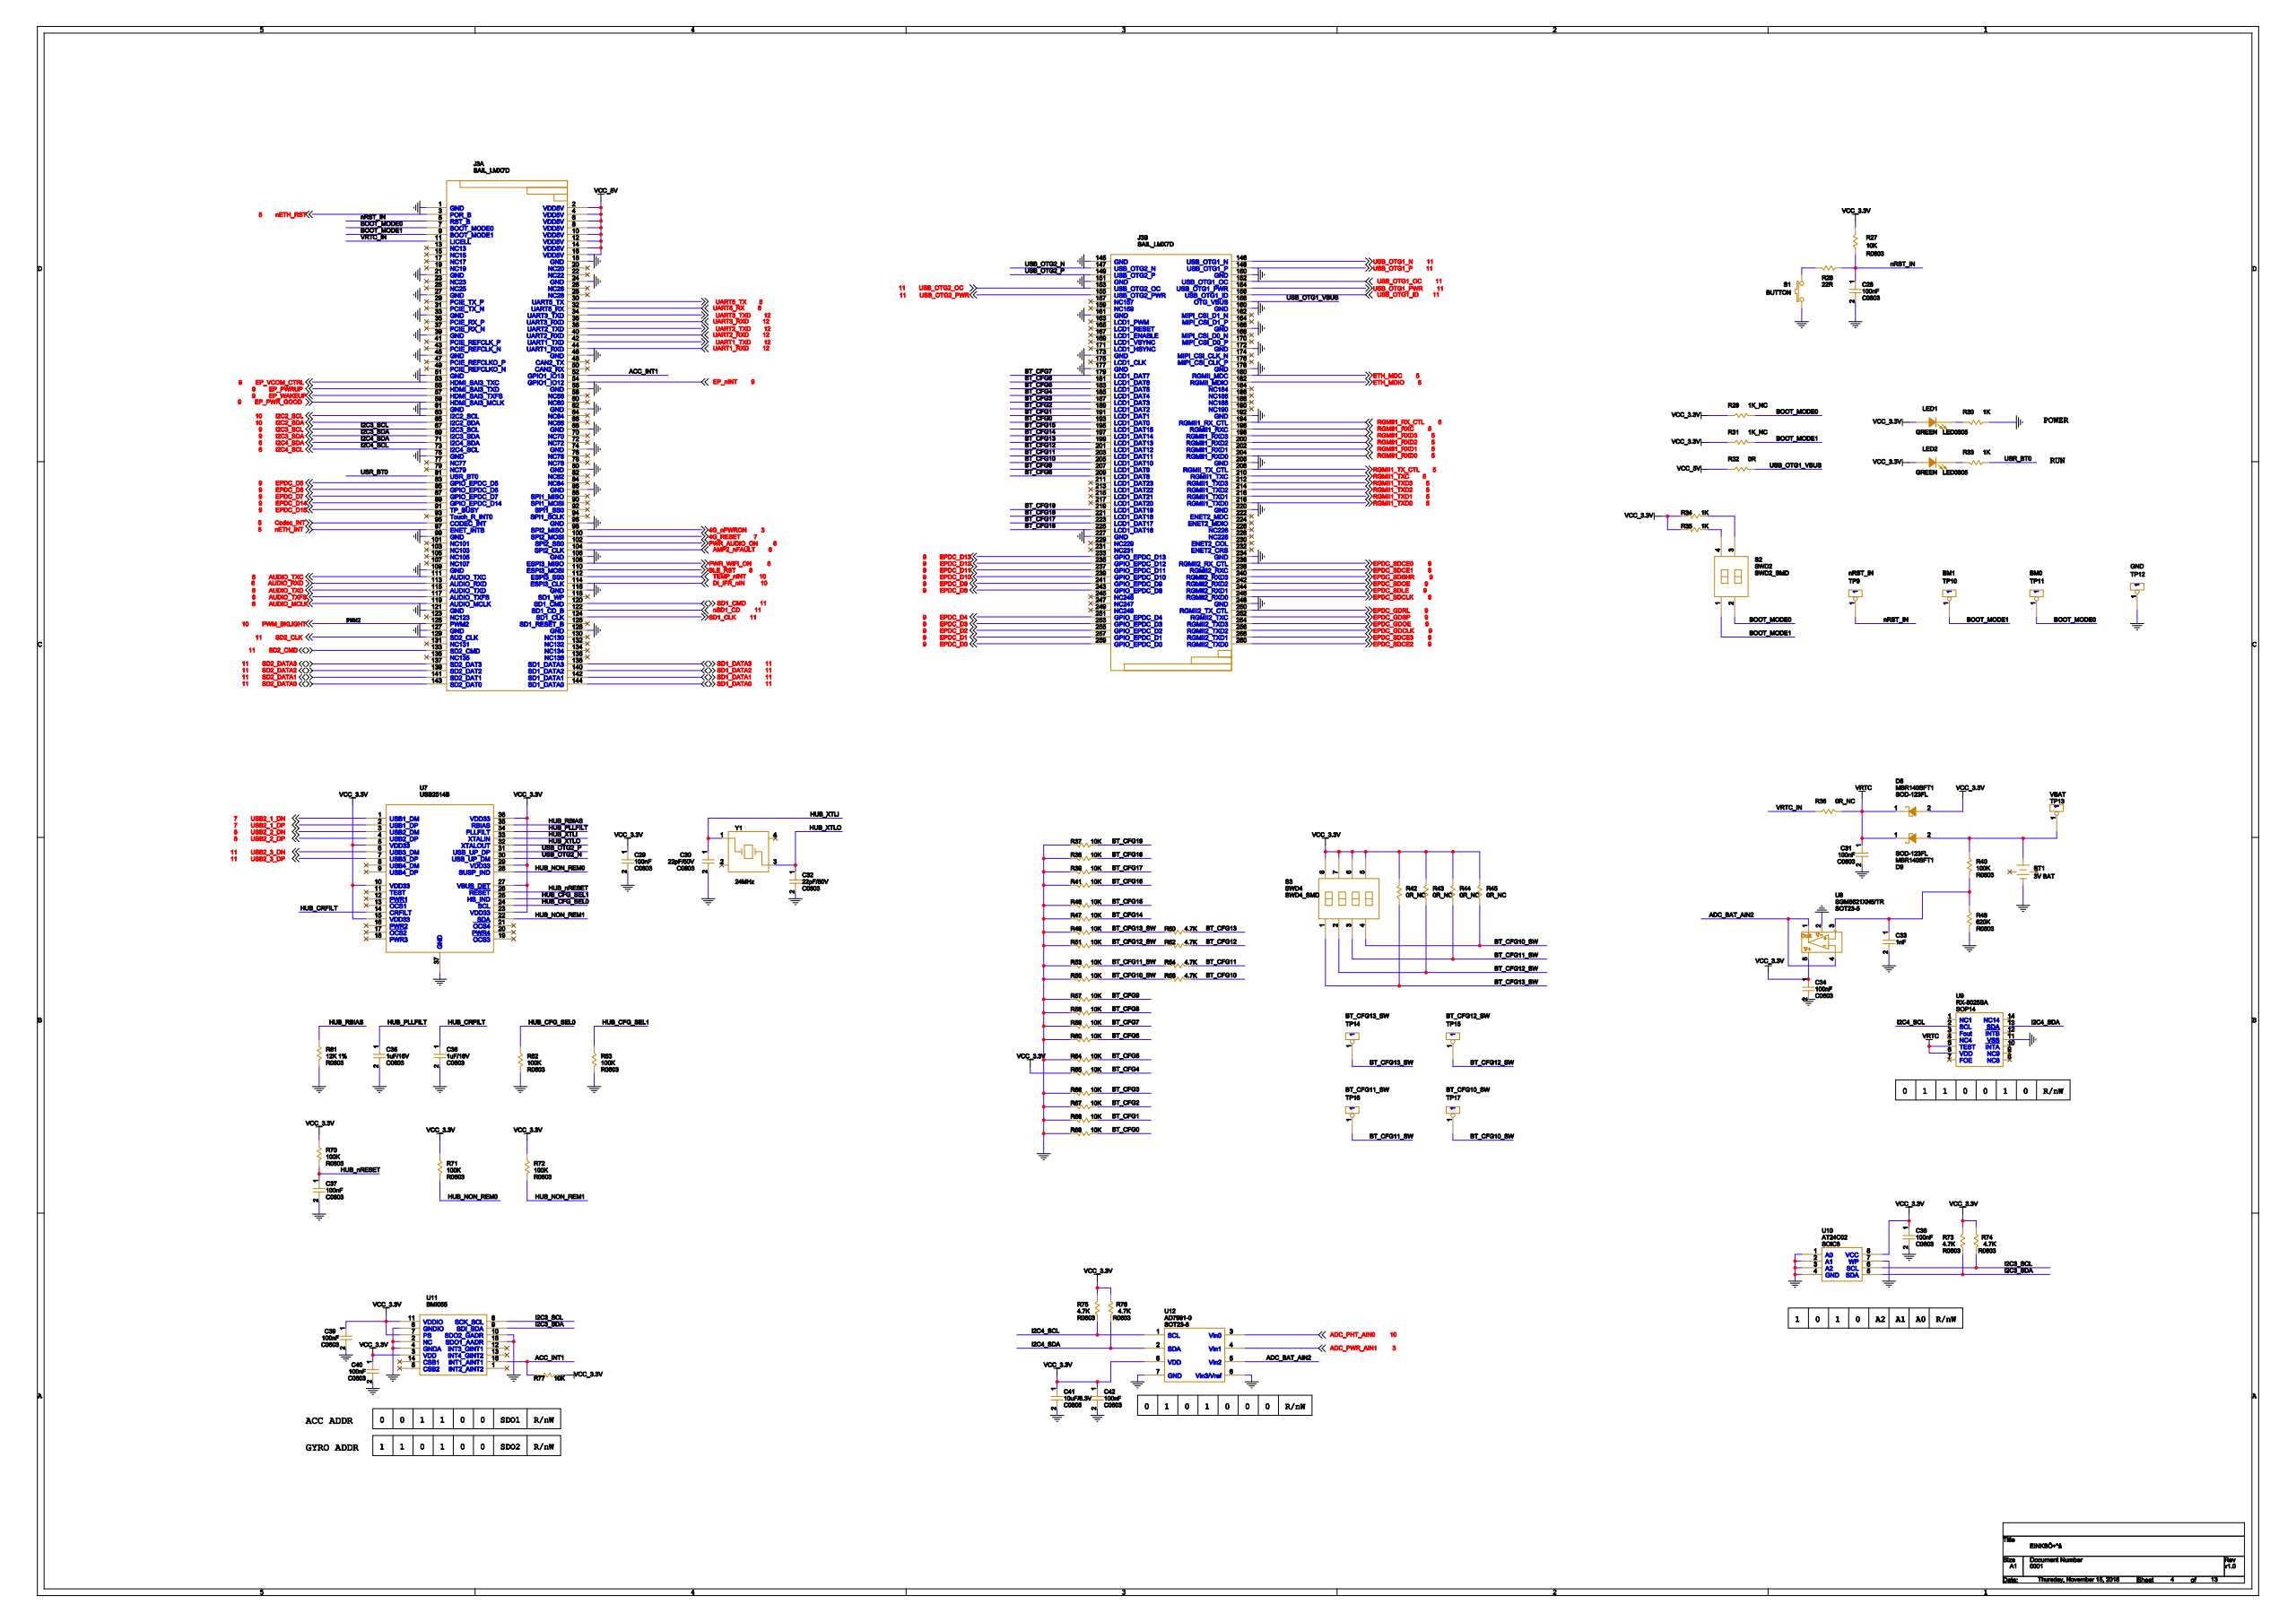Circuit board | Cadence Allegro | 609 parts | 409 nets | one sheet of the schematic
Parts on this sheet (reference | value | footprint):
BT1 | 3V BAT | BAT600
C28 | 100nF | C0603
C29 | 100nF | C0603
C30 | 22pF/50V | C0603
C31 | 100nF | C0603
C32 | 22pF/50V | C0603
C33 | 1nF | C0603
C34 | 100nF | C0603
C35 | 1uF/16V | C0603
C36 | 1uF/16V | C0603
C37 | 100nF | C0603
C38 | 100nF | C0603
C39 | 100nF | C0603
C40 | 100nF | C0603
C41 | 10uF/6.3V | C0805
C42 | 100nF | C0603
D8 | MBR140SFT1 | SOD-123FL
D9 | MBR140SFT1 | SOD-123FL
J3 | SAIL_i.MX7D | DDR4_SLT_RVS
LED1 | GREEN | LED0805
LED2 | GREEN | LED0805
R27 | 10K | R0603
R28 | 22R | R0603
R29 | 1K_NC | R0603
R30 | 1K | R0603
R31 | 1K_NC | R0603
R32 | 0R | R0603
R33 | 1K | R0603
R34 | 1K | R0603
R35 | 1K | R0603
R36 | 0R_NC | R0603
R37 | 10K | R0603
R38 | 10K | R0603
R39 | 10K | R0603
R40 | 100K | R0603
R41 | 10K | R0603
R42 | 0R_NC | R0603
R43 | 0R_NC | R0603
R44 | 0R_NC | R0603
R45 | 0R_NC | R0603
R46 | 10K | R0603
R47 | 10K | R0603
R48 | 620K | R0603
R49 | 10K | R0603
R50 | 4.7K | R0603
R51 | 10K | R0603
R52 | 4.7K | R0603
R53 | 10K | R0603
R54 | 4.7K | R0603
R55 | 10K | R0603
R56 | 4.7K | R0603
R57 | 10K | R0603
R58 | 10K | R0603
R59 | 10K | R0603
R60 | 10K | R0603
R61 | 12K 1% | R0603
R62 | 100K | R0603
R63 | 100K | R0603
R64 | 10K | R0603
R65 | 10K | R0603
R66 | 10K | R0603
R67 | 10K | R0603
R68 | 10K | R0603
R69 | 10K | R0603
R70 | 100K | R0603
R71 | 100K | R0603
R72 | 100K | R0603
R73 | 4.7K | R0603
R74 | 4.7K | R0603
R75 | 4.7K | R0603
R76 | 4.7K | R0603
R77 | 10K | R0603
S1 | BUTTON | BUTTON_4X6
S2 | SWD2 | SWD2_SMD
S3 | SWD4 | SWD4_SMD
TP9 | nRST_IN | TP_50
TP10 | BM1 | TP_50
TP11 | BM0 | TP_50
TP12 | GND | TP_50
TP13 | VBAT | TP_50
TP14 | BT_CFG13_SW | TP_50
TP15 | BT_CFG12_SW | TP_50
TP16 | BT_CFG11_SW | TP_50
TP17 | BT_CFG10_SW | TP_50
U7 | USB2514B | SQFN36
U9 | RX-8025SA | SOP14
U10 | AT24C02 | SOIC8
U11 | BMI055 | BMI055
U12 | AD7991-0 | SOT23-8
Y1 | 24MHz | XTAL4_SX_3225
Nets of these parts (net: part-pin ...):
GND: BT1-2 C28-2 C29-2 C30-2 C31-2 C32-2 C33-2 C34-2 C35-2 C36-2 C37-2 C38-2 C39-2 C40-2 C41-2 C42-2 R30-1 R37-2 R38-2 R39-2 R41-2 R46-2 R47-2 R48-1 R49-2 R51-2 R53-2 R55-2 R57-2 R58-2 R59-2 R60-2 R61-2 R62-1 R63-1 R64-2 R66-2 R67-2 R68-2 R69-2 S1-2 TP12-1 U9-11 U10-1 U10-2 U10-3 U10-4 U10-7 U11-2 U11-4 U11-6 U11-10 U11-15 U12-6 U12-7 J3-1 J3-18 J3-21 J3-24 J3-27 J3-33 J3-39 J3-45 J3-46 J3-51 J3-56 J3-61 J3-62 J3-68 J3-74 J3-75 J3-80 J3-86 J3-96 J3-99 J3-106 J3-109 J3-116 J3-121 J3-127 J3-128 J3-145 J3-150 J3-151 J3-160 J3-161 J3-166 J3-172 J3-173 J3-177 J3-178 J3-192 J3-206 J3-220 J3-227 J3-234 J3-248 U7-37
N28737094: BT1-1 D9-2 R40-2 TP13-1
VCC_3.3V: C29-1 C34-1 C38-1 C39-1 C40-1 C41-1 C42-1 D8-2 LED1-2 LED2-2 R27-2 R29-2 R31-2 R34-2 R35-2 R42-1 R43-1 R44-1 R45-1 R65-2 R70-2 R71-2 R72-2 R73-2 R74-2 R75-2 R76-2 R77-1 S3-5 S3-6 S3-7 S3-8 U10-8 U11-3 U11-7 U11-11 U12-8 U7-5 U7-10 U7-15 U7-23 U7-27 U7-29 U7-36
VCC_5V: R32-2 J3-2 J3-4 J3-6 J3-8 J3-10 J3-12 J3-14 J3-16
SD1_CMD: J3-120
SD1_DATA0: J3-144
SD1_DATA1: J3-142
SD1_DATA2: J3-140
SD1_DATA3: J3-138
AUDIO_MCLK: J3-119
AUDIO_RXD: J3-113
AUDIO_TXC: J3-111
AUDIO_TXD: J3-115
AUDIO_TXFS: J3-117
BOOT_MODE0: R29-1 S2-2 TP11-1 J3-7
BOOT_MODE1: R31-1 S2-1 TP10-1 J3-9
CODEC_INT: J3-95
PWR_WIFI_ON: J3-108
BLE_RST: J3-110
ACC_INT1: R77-2 U11-16 J3-52
EPDC_D14: J3-89
EPDC_D5: J3-83
EPDC_D6: J3-85
EPDC_D7: J3-87
EP_PWR_GOOD: J3-59
EP_VCOM_CTRL: J3-53
EP_PWRUP: J3-55
EP_WAKEUP: J3-57
I2C2_SCL: J3-63
I2C2_SDA: J3-65
I2C3_SCL: R74-1 U10-6 U11-8 J3-67
I2C3_SDA: R73-1 U10-5 U11-9 J3-69
I2C4_SCL: R75-1 U9-2 U12-1 J3-73
I2C4_SDA: R76-1 U9-13 U12-2 J3-71
VRTC_IN: R36-2 J3-11
PWM_BKLIGHT: J3-125
NRST_IN: C28-1 R27-1 R28-1 TP9-1 J3-5
SD1_CLK: J3-124
SD2_CLK: J3-129
SD2_CMD: J3-133
SD2_DATA0: J3-143
SD2_DATA1: J3-141
SD2_DATA2: J3-139
SD2_DATA3: J3-137
4G_RESET: J3-100
PWR_AUDIO_ON: J3-102
EPDC_D15: J3-91
UART1_RXD: J3-44
UART1_TXD: J3-42
UART2_RXD: J3-40
UART2_TXD: J3-38
UART3_RXD: J3-36
UART3_TXD: J3-34
UART5_RX: J3-32
UART5_TX: J3-30
USR_BT0: R33-1 J3-81
EPDC_D0: J3-259
EPDC_D1: J3-257
EPDC_D10: J3-239
EPDC_D11: J3-237
EPDC_D12: J3-235
EPDC_D13: J3-233
EPDC_D2: J3-255
EPDC_D3: J3-253
EPDC_D4: J3-251
EPDC_D8: J3-243
EPDC_D9: J3-241
BT_CFG0: R69-1 J3-193
BT_CFG1: R68-1 J3-191
BT_CFG10: R56-1 J3-205
BT_CFG11: R54-1 J3-203
BT_CFG12: R52-1 J3-201
BT_CFG13: R50-1 J3-199
BT_CFG14: R47-1 J3-197
BT_CFG15: R46-1 J3-195
BT_CFG16: R41-1 J3-225
BT_CFG17: R39-1 J3-223
BT_CFG18: R38-1 J3-221
BT_CFG19: R37-1 J3-219
BT_CFG2: R67-1 J3-189
BT_CFG3: R66-1 J3-187
BT_CFG4: R65-1 J3-185
BT_CFG5: R64-1 J3-183
BT_CFG6: R60-1 J3-181
BT_CFG7: R59-1 J3-179
BT_CFG8: R58-1 J3-209
BT_CFG9: R57-1 J3-207
USB_OTG1_VBUS: R32-1 J3-158
RGMII1_RXC: J3-196
RGMII1_RXD0: J3-204
RGMII1_RXD1: J3-202
RGMII1_RXD2: J3-200
RGMII1_RXD3: J3-198
RGMII1_RX_CTL: J3-194
RGMII1_TXC: J3-210
RGMII1_TXD0: J3-218
RGMII1_TXD1: J3-216
RGMII1_TXD2: J3-214
RGMII1_TXD3: J3-212
EPDC_SDCE1: J3-238
EPDC_SDCLK: J3-246
EPDC_SDLE: J3-244
EPDC_SDOE: J3-242
EPDC_SDSHR: J3-240
EPDC_SDCE0: J3-236
EPDC_GDSP: J3-252
EPDC_SDCE2: J3-260
EPDC_SDCE3: J3-258
EPDC_GDCLK: J3-256
EPDC_GDOE: J3-254
EPDC_GDRL: J3-250
ETH_MDC: J3-180
ETH_MDIO: J3-182
RGMII1_TX_CTL: J3-208
USB_OTG1_ID: J3-156
USB_OTG1_N: J3-146
USB_OTG1_OC: J3-152
USB_OTG1_P: J3-148
USB_OTG1_PWR: J3-154
USB_OTG2_N: J3-147 U7-30
USB_OTG2_OC: J3-153
USB_OTG2_P: J3-149 U7-31
USB_OTG2_PWR: J3-155
N29227737: R34-1 S2-3
N29227732: R35-1 S2-4
BT_CFG13_SW: R42-2 R49-1 R50-2 S3-1 TP14-1
BT_CFG12_SW: R43-2 R51-1 R52-2 S3-2 TP15-1
BT_CFG11_SW: R44-2 R53-1 R54-2 S3-3 TP16-1
BT_CFG10_SW: R45-2 R55-1 R56-2 S3-4 TP17-1
ADC_PHT_AIN0: U12-3
ADC_PWR_AIN1: U12-4
ADC_BAT_AIN2: U12-5
HUB_CRFILT: C36-1 U7-14
HUB_CFG_SEL1: R63-2 U7-25
HUB_PLLFILT: C35-1 U7-34
HUB_RBIAS: R61-1 U7-35
HUB_NRESET: C37-1 R70-1 U7-26
HUB_CFG_SEL0: R62-2 U7-24
HUB_NON_REM1: R72-1 U7-22
HUB_NON_REM0: R71-1 U7-28
USB2_1_DN: U7-1
USB2_1_DP: U7-2
USB2_2_DN: U7-3
USB2_2_DP: U7-4
USB2_3_DN: U7-6
USB2_3_DP: U7-7
HUB_XTLI: C30-1 Y1-1 U7-33
HUB_XTLO: C32-1 Y1-3 U7-32
N28737112: C33-1 R40-1 R48-2
VRTC: C31-1 D8-1 D9-1 R36-1 U9-5 U9-6
N28742261: LED1-1 R30-2
N28742366: LED2-1 R33-2
N28227382: R28-2 S1-1